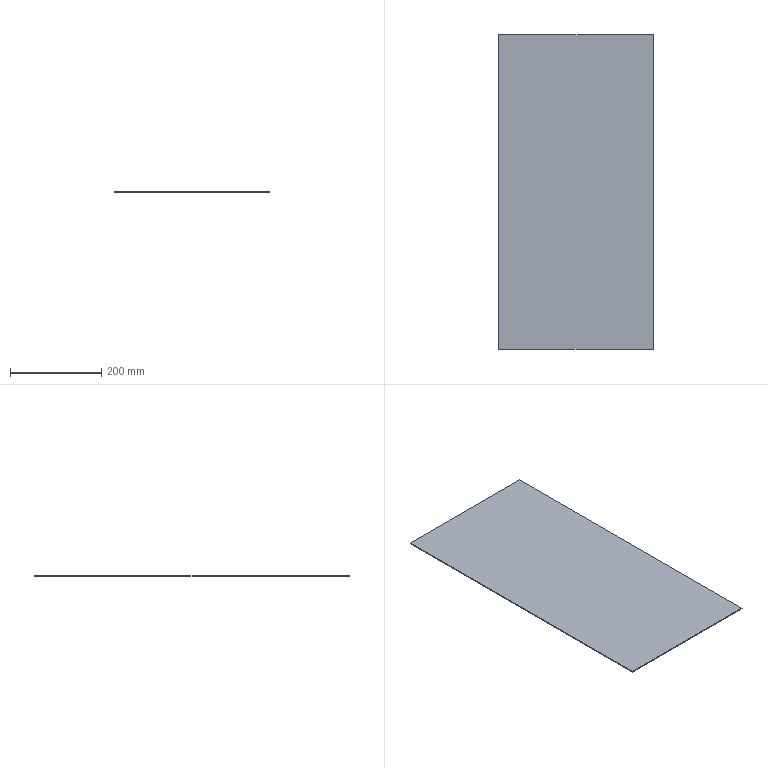Part | SolidWorks | features Extrusion 1 | 1 solid | 6 faces | box 340 x 690 x 2 mm | volume 469200 mm3 | plane 6
STEP:
#1=CARTESIAN_POINT('',(-251.402,170.884,0.));
#2=VERTEX_POINT('',#1);
#3=CARTESIAN_POINT('',(-251.402,-519.116,0.));
#4=VERTEX_POINT('',#3);
#5=CARTESIAN_POINT('',(-251.402,170.884,0.));
#6=DIRECTION('',(0.,-1.,0.));
#7=VECTOR('',#6,1000.);
#8=LINE('',#5,#7);
#9=EDGE_CURVE('',#2,#4,#8,.T.);
#10=ORIENTED_EDGE('',*,*,#9,.T.);
#11=CARTESIAN_POINT('',(-251.402,-519.116,2.));
#12=VERTEX_POINT('',#11);
#13=CARTESIAN_POINT('',(-251.402,-519.116,2.));
#14=DIRECTION('',(0.,0.,-1.));
#15=VECTOR('',#14,1000.);
#16=LINE('',#13,#15);
#17=EDGE_CURVE('',#12,#4,#16,.T.);
#18=ORIENTED_EDGE('',*,*,#17,.F.);
#19=CARTESIAN_POINT('',(-251.402,170.884,2.));
#20=VERTEX_POINT('',#19);
#21=CARTESIAN_POINT('',(-251.402,170.884,2.));
#22=DIRECTION('',(0.,-1.,0.));
#23=VECTOR('',#22,1000.);
#24=LINE('',#21,#23);
#25=EDGE_CURVE('',#20,#12,#24,.T.);
#26=ORIENTED_EDGE('',*,*,#25,.F.);
#27=CARTESIAN_POINT('',(-251.402,170.884,2.));
#28=DIRECTION('',(0.,0.,-1.));
#29=VECTOR('',#28,1000.);
#30=LINE('',#27,#29);
#31=EDGE_CURVE('',#20,#2,#30,.T.);
#32=ORIENTED_EDGE('',*,*,#31,.T.);
#33=EDGE_LOOP('',(#10,#18,#26,#32));
#34=FACE_OUTER_BOUND('',#33,.T.);
#35=CARTESIAN_POINT('',(-251.402,170.884,2.));
#36=DIRECTION('',(1.,0.,0.));
#37=DIRECTION('',(0.,1.,0.));
#38=AXIS2_PLACEMENT_3D('',#35,#36,#37);
#39=PLANE('',#38);
#40=ADVANCED_FACE('',(#34),#39,.F.);
#41=CARTESIAN_POINT('',(88.598,-519.116,0.));
#42=VERTEX_POINT('',#41);
#43=CARTESIAN_POINT('',(-251.402,-519.116,0.));
#44=DIRECTION('',(1.,0.,0.));
#45=VECTOR('',#44,1000.);
#46=LINE('',#43,#45);
#47=EDGE_CURVE('',#4,#42,#46,.T.);
#48=ORIENTED_EDGE('',*,*,#47,.T.);
#49=CARTESIAN_POINT('',(88.598,-519.116,2.));
#50=VERTEX_POINT('',#49);
#51=CARTESIAN_POINT('',(88.598,-519.116,2.));
#52=DIRECTION('',(0.,0.,-1.));
#53=VECTOR('',#52,1000.);
#54=LINE('',#51,#53);
#55=EDGE_CURVE('',#50,#42,#54,.T.);
#56=ORIENTED_EDGE('',*,*,#55,.F.);
#57=CARTESIAN_POINT('',(-251.402,-519.116,2.));
#58=DIRECTION('',(1.,0.,0.));
#59=VECTOR('',#58,1000.);
#60=LINE('',#57,#59);
#61=EDGE_CURVE('',#12,#50,#60,.T.);
#62=ORIENTED_EDGE('',*,*,#61,.F.);
#63=ORIENTED_EDGE('',*,*,#17,.T.);
#64=EDGE_LOOP('',(#48,#56,#62,#63));
#65=FACE_OUTER_BOUND('',#64,.T.);
#66=CARTESIAN_POINT('',(-251.402,-519.116,2.));
#67=DIRECTION('',(0.,1.,0.));
#68=DIRECTION('',(0.,0.,1.));
#69=AXIS2_PLACEMENT_3D('',#66,#67,#68);
#70=PLANE('',#69);
#71=ADVANCED_FACE('',(#65),#70,.F.);
#72=CARTESIAN_POINT('',(88.598,170.884,0.));
#73=VERTEX_POINT('',#72);
#74=CARTESIAN_POINT('',(88.598,170.884,0.));
#75=DIRECTION('',(0.,1.,0.));
#76=VECTOR('',#75,1000.);
#77=LINE('',#74,#76);
#78=EDGE_CURVE('',#42,#73,#77,.T.);
#79=ORIENTED_EDGE('',*,*,#78,.T.);
#80=CARTESIAN_POINT('',(88.598,170.884,2.));
#81=VERTEX_POINT('',#80);
#82=CARTESIAN_POINT('',(88.598,170.884,2.));
#83=DIRECTION('',(0.,0.,-1.));
#84=VECTOR('',#83,1000.);
#85=LINE('',#82,#84);
#86=EDGE_CURVE('',#81,#73,#85,.T.);
#87=ORIENTED_EDGE('',*,*,#86,.F.);
#88=CARTESIAN_POINT('',(88.598,170.884,2.));
#89=DIRECTION('',(0.,1.,0.));
#90=VECTOR('',#89,1000.);
#91=LINE('',#88,#90);
#92=EDGE_CURVE('',#50,#81,#91,.T.);
#93=ORIENTED_EDGE('',*,*,#92,.F.);
#94=ORIENTED_EDGE('',*,*,#55,.T.);
#95=EDGE_LOOP('',(#79,#87,#93,#94));
#96=FACE_OUTER_BOUND('',#95,.T.);
#97=CARTESIAN_POINT('',(88.598,170.884,2.));
#98=DIRECTION('',(-1.,0.,0.));
#99=DIRECTION('',(0.,-1.,0.));
#100=AXIS2_PLACEMENT_3D('',#97,#98,#99);
#101=PLANE('',#100);
#102=ADVANCED_FACE('',(#96),#101,.F.);
#103=CARTESIAN_POINT('',(-251.402,170.884,0.));
#104=DIRECTION('',(-1.,0.,0.));
#105=VECTOR('',#104,1000.);
#106=LINE('',#103,#105);
#107=EDGE_CURVE('',#73,#2,#106,.T.);
#108=ORIENTED_EDGE('',*,*,#107,.T.);
#109=ORIENTED_EDGE('',*,*,#31,.F.);
#110=CARTESIAN_POINT('',(-251.402,170.884,2.));
#111=DIRECTION('',(-1.,0.,0.));
#112=VECTOR('',#111,1000.);
#113=LINE('',#110,#112);
#114=EDGE_CURVE('',#81,#20,#113,.T.);
#115=ORIENTED_EDGE('',*,*,#114,.F.);
#116=ORIENTED_EDGE('',*,*,#86,.T.);
#117=EDGE_LOOP('',(#108,#109,#115,#116));
#118=FACE_OUTER_BOUND('',#117,.T.);
#119=CARTESIAN_POINT('',(-251.402,170.884,2.));
#120=DIRECTION('',(0.,-1.,0.));
#121=DIRECTION('',(0.,0.,-1.));
#122=AXIS2_PLACEMENT_3D('',#119,#120,#121);
#123=PLANE('',#122);
#124=ADVANCED_FACE('',(#118),#123,.F.);
#125=ORIENTED_EDGE('',*,*,#25,.T.);
#126=ORIENTED_EDGE('',*,*,#61,.T.);
#127=ORIENTED_EDGE('',*,*,#92,.T.);
#128=ORIENTED_EDGE('',*,*,#114,.T.);
#129=EDGE_LOOP('',(#125,#126,#127,#128));
#130=FACE_OUTER_BOUND('',#129,.T.);
#131=CARTESIAN_POINT('',(0.,0.,2.));
#132=DIRECTION('',(0.,0.,1.));
#133=DIRECTION('',(1.,0.,0.));
#134=AXIS2_PLACEMENT_3D('',#131,#132,#133);
#135=PLANE('',#134);
#136=ADVANCED_FACE('',(#130),#135,.T.);
#137=ORIENTED_EDGE('',*,*,#9,.F.);
#138=ORIENTED_EDGE('',*,*,#107,.F.);
#139=ORIENTED_EDGE('',*,*,#78,.F.);
#140=ORIENTED_EDGE('',*,*,#47,.F.);
#141=EDGE_LOOP('',(#137,#138,#139,#140));
#142=FACE_OUTER_BOUND('',#141,.T.);
#143=CARTESIAN_POINT('',(0.,0.,0.));
#144=DIRECTION('',(0.,0.,1.));
#145=DIRECTION('',(1.,0.,0.));
#146=AXIS2_PLACEMENT_3D('',#143,#144,#145);
#147=PLANE('',#146);
#148=ADVANCED_FACE('',(#142),#147,.F.);
#149=CLOSED_SHELL('',(#40,#71,#102,#124,#136,#148));
#150=MANIFOLD_SOLID_BREP('',#149);
#151=CARTESIAN_POINT('',(0.,0.,0.));
#152=DIRECTION('',(0.,0.,1.));
#153=DIRECTION('',(1.,0.,0.));
#154=AXIS2_PLACEMENT_3D('',#151,#152,#153);
#155=(LENGTH_UNIT()NAMED_UNIT(*)SI_UNIT(.MILLI.,.METRE.));
#156=UNCERTAINTY_MEASURE_WITH_UNIT(LENGTH_MEASURE(0.00001),#155,'','');
#157=(NAMED_UNIT(*)PLANE_ANGLE_UNIT()SI_UNIT($,.RADIAN.));
#158=(NAMED_UNIT(*)SI_UNIT($,.STERADIAN.)SOLID_ANGLE_UNIT());
#159=(GEOMETRIC_REPRESENTATION_CONTEXT(3)GLOBAL_UNCERTAINTY_ASSIGNED_CONTEXT((#156))GLOBAL_UNIT_ASSIGNED_CONTEXT((#155,#157,#158))REPRESENTATION_CONTEXT('',''));
#160=ADVANCED_BREP_SHAPE_REPRESENTATION('',(#150,#154),#159);